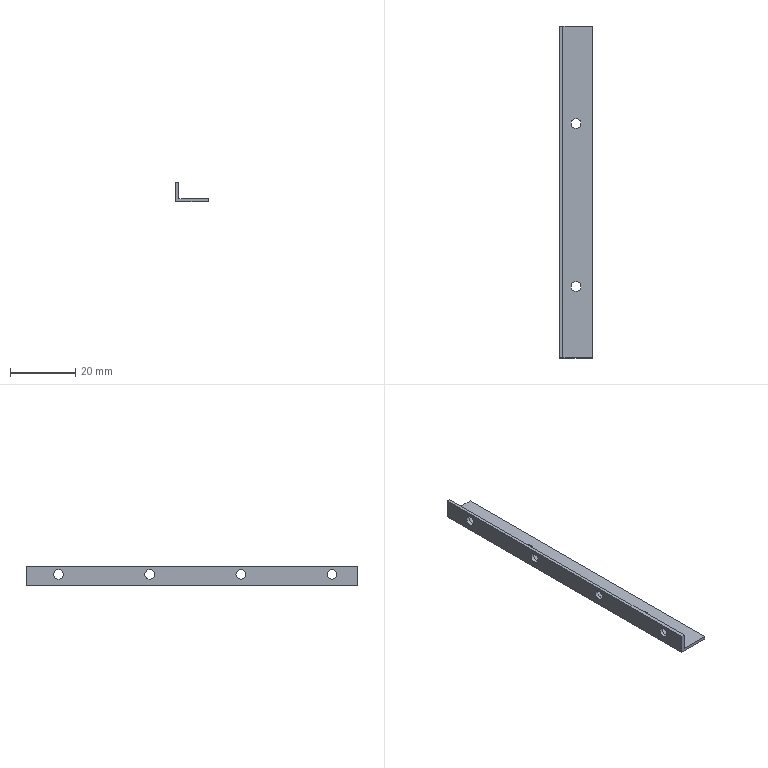Part | STEP file | 1-31.2 | 1 solid | 14 faces | box 10 x 102 x 6 mm | volume 1488 mm3 | plane 8 | cylinder 6 | commonest cylinder face diameters 3 x6
STEP:
#1=CARTESIAN_POINT('',(0.,0.,0.));
#2=DIRECTION('',(0.,0.,1.));
#3=DIRECTION('',(1.,0.,0.));
#4=AXIS2_PLACEMENT_3D('',#1,#2,#3);
#5=CARTESIAN_POINT('',(0.,-51.,0.));
#6=VERTEX_POINT('',#5);
#7=CARTESIAN_POINT('',(10.,-51.,0.));
#8=VERTEX_POINT('',#7);
#9=CARTESIAN_POINT('',(0.,-51.,0.));
#10=DIRECTION('',(1.,0.,0.));
#11=VECTOR('',#10,1.);
#12=LINE('',#9,#11);
#13=CARTESIAN_POINT('',(5.,-51.,5.));
#14=DIRECTION('',(0.,-1.,0.));
#15=DIRECTION('',(1.,0.,0.));
#16=AXIS2_PLACEMENT_3D('',#13,#14,#15);
#17=PLANE('',#16);
#18=CARTESIAN_POINT('',(-5.,-5.));
#19=DIRECTION('',(1.,0.));
#20=VECTOR('',#19,1.);
#21=LINE('',#18,#20);
#22=(GEOMETRIC_REPRESENTATION_CONTEXT(2)PARAMETRIC_REPRESENTATION_CONTEXT()REPRESENTATION_CONTEXT('',''));
#23=DEFINITIONAL_REPRESENTATION('',(#21),#22);
#24=PCURVE('',#17,#23);
#25=CARTESIAN_POINT('',(5.,0.,0.));
#26=DIRECTION('',(0.,0.,1.));
#27=DIRECTION('',(1.,0.,0.));
#28=AXIS2_PLACEMENT_3D('',#25,#26,#27);
#29=PLANE('',#28);
#30=CARTESIAN_POINT('',(-5.,-51.));
#31=DIRECTION('',(1.,0.));
#32=VECTOR('',#31,1.);
#33=LINE('',#30,#32);
#34=(GEOMETRIC_REPRESENTATION_CONTEXT(2)PARAMETRIC_REPRESENTATION_CONTEXT()REPRESENTATION_CONTEXT('',''));
#35=DEFINITIONAL_REPRESENTATION('',(#33),#34);
#36=PCURVE('',#29,#35);
#37=SURFACE_CURVE('',#12,(#24,#36),.PCURVE_S1.);
#38=EDGE_CURVE('',#6,#8,#37,.T.);
#39=ORIENTED_EDGE('',*,*,#38,.T.);
#40=CARTESIAN_POINT('',(10.,-51.,1.));
#41=VERTEX_POINT('',#40);
#42=CARTESIAN_POINT('',(10.,-51.,0.));
#43=DIRECTION('',(0.,0.,1.));
#44=VECTOR('',#43,1.);
#45=LINE('',#42,#44);
#46=CARTESIAN_POINT('',(5.,-5.));
#47=DIRECTION('',(0.,1.));
#48=VECTOR('',#47,1.);
#49=LINE('',#46,#48);
#50=(GEOMETRIC_REPRESENTATION_CONTEXT(2)PARAMETRIC_REPRESENTATION_CONTEXT()REPRESENTATION_CONTEXT('',''));
#51=DEFINITIONAL_REPRESENTATION('',(#49),#50);
#52=PCURVE('',#17,#51);
#53=CARTESIAN_POINT('',(10.,0.,0.5));
#54=DIRECTION('',(-1.,0.,0.));
#55=DIRECTION('',(0.,0.,1.));
#56=AXIS2_PLACEMENT_3D('',#53,#54,#55);
#57=PLANE('',#56);
#58=CARTESIAN_POINT('',(-0.5,-51.));
#59=DIRECTION('',(1.,0.));
#60=VECTOR('',#59,1.);
#61=LINE('',#58,#60);
#62=(GEOMETRIC_REPRESENTATION_CONTEXT(2)PARAMETRIC_REPRESENTATION_CONTEXT()REPRESENTATION_CONTEXT('',''));
#63=DEFINITIONAL_REPRESENTATION('',(#61),#62);
#64=PCURVE('',#57,#63);
#65=SURFACE_CURVE('',#45,(#52,#64),.PCURVE_S1.);
#66=EDGE_CURVE('',#8,#41,#65,.T.);
#67=ORIENTED_EDGE('',*,*,#66,.T.);
#68=CARTESIAN_POINT('',(1.,-51.,1.));
#69=VERTEX_POINT('',#68);
#70=CARTESIAN_POINT('',(10.,-51.,1.));
#71=DIRECTION('',(-1.,0.,0.));
#72=VECTOR('',#71,1.);
#73=LINE('',#70,#72);
#74=CARTESIAN_POINT('',(5.,-4.));
#75=DIRECTION('',(-1.,0.));
#76=VECTOR('',#75,1.);
#77=LINE('',#74,#76);
#78=(GEOMETRIC_REPRESENTATION_CONTEXT(2)PARAMETRIC_REPRESENTATION_CONTEXT()REPRESENTATION_CONTEXT('',''));
#79=DEFINITIONAL_REPRESENTATION('',(#77),#78);
#80=PCURVE('',#17,#79);
#81=CARTESIAN_POINT('',(5.5,0.,1.));
#82=DIRECTION('',(0.,0.,-1.));
#83=DIRECTION('',(-1.,0.,0.));
#84=AXIS2_PLACEMENT_3D('',#81,#82,#83);
#85=PLANE('',#84);
#86=CARTESIAN_POINT('',(-4.5,-51.));
#87=DIRECTION('',(1.,0.));
#88=VECTOR('',#87,1.);
#89=LINE('',#86,#88);
#90=(GEOMETRIC_REPRESENTATION_CONTEXT(2)PARAMETRIC_REPRESENTATION_CONTEXT()REPRESENTATION_CONTEXT('',''));
#91=DEFINITIONAL_REPRESENTATION('',(#89),#90);
#92=PCURVE('',#85,#91);
#93=SURFACE_CURVE('',#73,(#80,#92),.PCURVE_S1.);
#94=EDGE_CURVE('',#41,#69,#93,.T.);
#95=ORIENTED_EDGE('',*,*,#94,.T.);
#96=CARTESIAN_POINT('',(1.,-51.,6.));
#97=VERTEX_POINT('',#96);
#98=CARTESIAN_POINT('',(1.,-51.,1.));
#99=DIRECTION('',(0.,0.,1.));
#100=VECTOR('',#99,1.);
#101=LINE('',#98,#100);
#102=CARTESIAN_POINT('',(-4.,-4.));
#103=DIRECTION('',(0.,1.));
#104=VECTOR('',#103,1.);
#105=LINE('',#102,#104);
#106=(GEOMETRIC_REPRESENTATION_CONTEXT(2)PARAMETRIC_REPRESENTATION_CONTEXT()REPRESENTATION_CONTEXT('',''));
#107=DEFINITIONAL_REPRESENTATION('',(#105),#106);
#108=PCURVE('',#17,#107);
#109=CARTESIAN_POINT('',(1.,0.,3.5));
#110=DIRECTION('',(-1.,0.,0.));
#111=DIRECTION('',(0.,0.,1.));
#112=AXIS2_PLACEMENT_3D('',#109,#110,#111);
#113=PLANE('',#112);
#114=CARTESIAN_POINT('',(-2.5,-51.));
#115=DIRECTION('',(1.,0.));
#116=VECTOR('',#115,1.);
#117=LINE('',#114,#116);
#118=(GEOMETRIC_REPRESENTATION_CONTEXT(2)PARAMETRIC_REPRESENTATION_CONTEXT()REPRESENTATION_CONTEXT('',''));
#119=DEFINITIONAL_REPRESENTATION('',(#117),#118);
#120=PCURVE('',#113,#119);
#121=SURFACE_CURVE('',#101,(#108,#120),.PCURVE_S1.);
#122=EDGE_CURVE('',#69,#97,#121,.T.);
#123=ORIENTED_EDGE('',*,*,#122,.T.);
#124=CARTESIAN_POINT('',(0.,-51.,6.));
#125=VERTEX_POINT('',#124);
#126=CARTESIAN_POINT('',(1.,-51.,6.));
#127=DIRECTION('',(-1.,0.,0.));
#128=VECTOR('',#127,1.);
#129=LINE('',#126,#128);
#130=CARTESIAN_POINT('',(-4.,1.));
#131=DIRECTION('',(-1.,0.));
#132=VECTOR('',#131,1.);
#133=LINE('',#130,#132);
#134=(GEOMETRIC_REPRESENTATION_CONTEXT(2)PARAMETRIC_REPRESENTATION_CONTEXT()REPRESENTATION_CONTEXT('',''));
#135=DEFINITIONAL_REPRESENTATION('',(#133),#134);
#136=PCURVE('',#17,#135);
#137=CARTESIAN_POINT('',(0.5,0.,6.));
#138=DIRECTION('',(0.,0.,-1.));
#139=DIRECTION('',(-1.,0.,0.));
#140=AXIS2_PLACEMENT_3D('',#137,#138,#139);
#141=PLANE('',#140);
#142=CARTESIAN_POINT('',(-0.5,-51.));
#143=DIRECTION('',(1.,0.));
#144=VECTOR('',#143,1.);
#145=LINE('',#142,#144);
#146=(GEOMETRIC_REPRESENTATION_CONTEXT(2)PARAMETRIC_REPRESENTATION_CONTEXT()REPRESENTATION_CONTEXT('',''));
#147=DEFINITIONAL_REPRESENTATION('',(#145),#146);
#148=PCURVE('',#141,#147);
#149=SURFACE_CURVE('',#129,(#136,#148),.PCURVE_S1.);
#150=EDGE_CURVE('',#97,#125,#149,.T.);
#151=ORIENTED_EDGE('',*,*,#150,.T.);
#152=CARTESIAN_POINT('',(0.,-51.,6.));
#153=DIRECTION('',(0.,0.,-1.));
#154=VECTOR('',#153,1.);
#155=LINE('',#152,#154);
#156=CARTESIAN_POINT('',(-5.,1.));
#157=DIRECTION('',(0.,-1.));
#158=VECTOR('',#157,1.);
#159=LINE('',#156,#158);
#160=(GEOMETRIC_REPRESENTATION_CONTEXT(2)PARAMETRIC_REPRESENTATION_CONTEXT()REPRESENTATION_CONTEXT('',''));
#161=DEFINITIONAL_REPRESENTATION('',(#159),#160);
#162=PCURVE('',#17,#161);
#163=CARTESIAN_POINT('',(0.,0.,3.));
#164=DIRECTION('',(1.,0.,0.));
#165=DIRECTION('',(0.,0.,-1.));
#166=AXIS2_PLACEMENT_3D('',#163,#164,#165);
#167=PLANE('',#166);
#168=CARTESIAN_POINT('',(-3.,-51.));
#169=DIRECTION('',(1.,0.));
#170=VECTOR('',#169,1.);
#171=LINE('',#168,#170);
#172=(GEOMETRIC_REPRESENTATION_CONTEXT(2)PARAMETRIC_REPRESENTATION_CONTEXT()REPRESENTATION_CONTEXT('',''));
#173=DEFINITIONAL_REPRESENTATION('',(#171),#172);
#174=PCURVE('',#167,#173);
#175=SURFACE_CURVE('',#155,(#162,#174),.PCURVE_S1.);
#176=EDGE_CURVE('',#125,#6,#175,.T.);
#177=ORIENTED_EDGE('',*,*,#176,.T.);
#178=EDGE_LOOP('',(#39,#67,#95,#123,#151,#177));
#179=FACE_BOUND('',#178,.T.);
#180=ADVANCED_FACE('',(#179),#17,.T.);
#181=CARTESIAN_POINT('',(0.,51.,0.));
#182=VERTEX_POINT('',#181);
#183=CARTESIAN_POINT('',(10.,51.,0.));
#184=VERTEX_POINT('',#183);
#185=CARTESIAN_POINT('',(0.,51.,0.));
#186=DIRECTION('',(1.,0.,0.));
#187=VECTOR('',#186,1.);
#188=LINE('',#185,#187);
#189=CARTESIAN_POINT('',(5.,51.,5.));
#190=DIRECTION('',(0.,-1.,0.));
#191=DIRECTION('',(1.,0.,0.));
#192=AXIS2_PLACEMENT_3D('',#189,#190,#191);
#193=PLANE('',#192);
#194=CARTESIAN_POINT('',(-5.,-5.));
#195=DIRECTION('',(1.,0.));
#196=VECTOR('',#195,1.);
#197=LINE('',#194,#196);
#198=(GEOMETRIC_REPRESENTATION_CONTEXT(2)PARAMETRIC_REPRESENTATION_CONTEXT()REPRESENTATION_CONTEXT('',''));
#199=DEFINITIONAL_REPRESENTATION('',(#197),#198);
#200=PCURVE('',#193,#199);
#201=CARTESIAN_POINT('',(-5.,51.));
#202=DIRECTION('',(1.,0.));
#203=VECTOR('',#202,1.);
#204=LINE('',#201,#203);
#205=(GEOMETRIC_REPRESENTATION_CONTEXT(2)PARAMETRIC_REPRESENTATION_CONTEXT()REPRESENTATION_CONTEXT('',''));
#206=DEFINITIONAL_REPRESENTATION('',(#204),#205);
#207=PCURVE('',#29,#206);
#208=SURFACE_CURVE('',#188,(#200,#207),.PCURVE_S1.);
#209=EDGE_CURVE('',#182,#184,#208,.T.);
#210=ORIENTED_EDGE('',*,*,#209,.T.);
#211=CARTESIAN_POINT('',(10.,51.,1.));
#212=VERTEX_POINT('',#211);
#213=CARTESIAN_POINT('',(10.,51.,0.));
#214=DIRECTION('',(0.,0.,1.));
#215=VECTOR('',#214,1.);
#216=LINE('',#213,#215);
#217=CARTESIAN_POINT('',(5.,-5.));
#218=DIRECTION('',(0.,1.));
#219=VECTOR('',#218,1.);
#220=LINE('',#217,#219);
#221=(GEOMETRIC_REPRESENTATION_CONTEXT(2)PARAMETRIC_REPRESENTATION_CONTEXT()REPRESENTATION_CONTEXT('',''));
#222=DEFINITIONAL_REPRESENTATION('',(#220),#221);
#223=PCURVE('',#193,#222);
#224=CARTESIAN_POINT('',(-0.5,51.));
#225=DIRECTION('',(1.,0.));
#226=VECTOR('',#225,1.);
#227=LINE('',#224,#226);
#228=(GEOMETRIC_REPRESENTATION_CONTEXT(2)PARAMETRIC_REPRESENTATION_CONTEXT()REPRESENTATION_CONTEXT('',''));
#229=DEFINITIONAL_REPRESENTATION('',(#227),#228);
#230=PCURVE('',#57,#229);
#231=SURFACE_CURVE('',#216,(#223,#230),.PCURVE_S1.);
#232=EDGE_CURVE('',#184,#212,#231,.T.);
#233=ORIENTED_EDGE('',*,*,#232,.T.);
#234=CARTESIAN_POINT('',(1.,51.,1.));
#235=VERTEX_POINT('',#234);
#236=CARTESIAN_POINT('',(10.,51.,1.));
#237=DIRECTION('',(-1.,0.,0.));
#238=VECTOR('',#237,1.);
#239=LINE('',#236,#238);
#240=CARTESIAN_POINT('',(5.,-4.));
#241=DIRECTION('',(-1.,0.));
#242=VECTOR('',#241,1.);
#243=LINE('',#240,#242);
#244=(GEOMETRIC_REPRESENTATION_CONTEXT(2)PARAMETRIC_REPRESENTATION_CONTEXT()REPRESENTATION_CONTEXT('',''));
#245=DEFINITIONAL_REPRESENTATION('',(#243),#244);
#246=PCURVE('',#193,#245);
#247=CARTESIAN_POINT('',(-4.5,51.));
#248=DIRECTION('',(1.,0.));
#249=VECTOR('',#248,1.);
#250=LINE('',#247,#249);
#251=(GEOMETRIC_REPRESENTATION_CONTEXT(2)PARAMETRIC_REPRESENTATION_CONTEXT()REPRESENTATION_CONTEXT('',''));
#252=DEFINITIONAL_REPRESENTATION('',(#250),#251);
#253=PCURVE('',#85,#252);
#254=SURFACE_CURVE('',#239,(#246,#253),.PCURVE_S1.);
#255=EDGE_CURVE('',#212,#235,#254,.T.);
#256=ORIENTED_EDGE('',*,*,#255,.T.);
#257=CARTESIAN_POINT('',(1.,51.,6.));
#258=VERTEX_POINT('',#257);
#259=CARTESIAN_POINT('',(1.,51.,1.));
#260=DIRECTION('',(0.,0.,1.));
#261=VECTOR('',#260,1.);
#262=LINE('',#259,#261);
#263=CARTESIAN_POINT('',(-4.,-4.));
#264=DIRECTION('',(0.,1.));
#265=VECTOR('',#264,1.);
#266=LINE('',#263,#265);
#267=(GEOMETRIC_REPRESENTATION_CONTEXT(2)PARAMETRIC_REPRESENTATION_CONTEXT()REPRESENTATION_CONTEXT('',''));
#268=DEFINITIONAL_REPRESENTATION('',(#266),#267);
#269=PCURVE('',#193,#268);
#270=CARTESIAN_POINT('',(-2.5,51.));
#271=DIRECTION('',(1.,0.));
#272=VECTOR('',#271,1.);
#273=LINE('',#270,#272);
#274=(GEOMETRIC_REPRESENTATION_CONTEXT(2)PARAMETRIC_REPRESENTATION_CONTEXT()REPRESENTATION_CONTEXT('',''));
#275=DEFINITIONAL_REPRESENTATION('',(#273),#274);
#276=PCURVE('',#113,#275);
#277=SURFACE_CURVE('',#262,(#269,#276),.PCURVE_S1.);
#278=EDGE_CURVE('',#235,#258,#277,.T.);
#279=ORIENTED_EDGE('',*,*,#278,.T.);
#280=CARTESIAN_POINT('',(0.,51.,6.));
#281=VERTEX_POINT('',#280);
#282=CARTESIAN_POINT('',(1.,51.,6.));
#283=DIRECTION('',(-1.,0.,0.));
#284=VECTOR('',#283,1.);
#285=LINE('',#282,#284);
#286=CARTESIAN_POINT('',(-4.,1.));
#287=DIRECTION('',(-1.,0.));
#288=VECTOR('',#287,1.);
#289=LINE('',#286,#288);
#290=(GEOMETRIC_REPRESENTATION_CONTEXT(2)PARAMETRIC_REPRESENTATION_CONTEXT()REPRESENTATION_CONTEXT('',''));
#291=DEFINITIONAL_REPRESENTATION('',(#289),#290);
#292=PCURVE('',#193,#291);
#293=CARTESIAN_POINT('',(-0.5,51.));
#294=DIRECTION('',(1.,0.));
#295=VECTOR('',#294,1.);
#296=LINE('',#293,#295);
#297=(GEOMETRIC_REPRESENTATION_CONTEXT(2)PARAMETRIC_REPRESENTATION_CONTEXT()REPRESENTATION_CONTEXT('',''));
#298=DEFINITIONAL_REPRESENTATION('',(#296),#297);
#299=PCURVE('',#141,#298);
#300=SURFACE_CURVE('',#285,(#292,#299),.PCURVE_S1.);
#301=EDGE_CURVE('',#258,#281,#300,.T.);
#302=ORIENTED_EDGE('',*,*,#301,.T.);
#303=CARTESIAN_POINT('',(0.,51.,6.));
#304=DIRECTION('',(0.,0.,-1.));
#305=VECTOR('',#304,1.);
#306=LINE('',#303,#305);
#307=CARTESIAN_POINT('',(-5.,1.));
#308=DIRECTION('',(0.,-1.));
#309=VECTOR('',#308,1.);
#310=LINE('',#307,#309);
#311=(GEOMETRIC_REPRESENTATION_CONTEXT(2)PARAMETRIC_REPRESENTATION_CONTEXT()REPRESENTATION_CONTEXT('',''));
#312=DEFINITIONAL_REPRESENTATION('',(#310),#311);
#313=PCURVE('',#193,#312);
#314=CARTESIAN_POINT('',(-3.,51.));
#315=DIRECTION('',(1.,0.));
#316=VECTOR('',#315,1.);
#317=LINE('',#314,#316);
#318=(GEOMETRIC_REPRESENTATION_CONTEXT(2)PARAMETRIC_REPRESENTATION_CONTEXT()REPRESENTATION_CONTEXT('',''));
#319=DEFINITIONAL_REPRESENTATION('',(#317),#318);
#320=PCURVE('',#167,#319);
#321=SURFACE_CURVE('',#306,(#313,#320),.PCURVE_S1.);
#322=EDGE_CURVE('',#281,#182,#321,.T.);
#323=ORIENTED_EDGE('',*,*,#322,.T.);
#324=EDGE_LOOP('',(#210,#233,#256,#279,#302,#323));
#325=FACE_BOUND('',#324,.F.);
#326=ADVANCED_FACE('',(#325),#193,.F.);
#327=ORIENTED_EDGE('',*,*,#66,.T.);
#328=CARTESIAN_POINT('',(10.,-51.,1.));
#329=DIRECTION('',(0.,1.,0.));
#330=VECTOR('',#329,1.);
#331=LINE('',#328,#330);
#332=CARTESIAN_POINT('',(0.5,-51.));
#333=DIRECTION('',(0.,1.));
#334=VECTOR('',#333,1.);
#335=LINE('',#332,#334);
#336=(GEOMETRIC_REPRESENTATION_CONTEXT(2)PARAMETRIC_REPRESENTATION_CONTEXT()REPRESENTATION_CONTEXT('',''));
#337=DEFINITIONAL_REPRESENTATION('',(#335),#336);
#338=PCURVE('',#57,#337);
#339=CARTESIAN_POINT('',(-4.5,-51.));
#340=DIRECTION('',(0.,1.));
#341=VECTOR('',#340,1.);
#342=LINE('',#339,#341);
#343=(GEOMETRIC_REPRESENTATION_CONTEXT(2)PARAMETRIC_REPRESENTATION_CONTEXT()REPRESENTATION_CONTEXT('',''));
#344=DEFINITIONAL_REPRESENTATION('',(#342),#343);
#345=PCURVE('',#85,#344);
#346=SURFACE_CURVE('',#331,(#338,#345),.PCURVE_S1.);
#347=EDGE_CURVE('',#41,#212,#346,.T.);
#348=ORIENTED_EDGE('',*,*,#347,.T.);
#349=ORIENTED_EDGE('',*,*,#232,.F.);
#350=CARTESIAN_POINT('',(10.,-51.,0.));
#351=DIRECTION('',(0.,1.,0.));
#352=VECTOR('',#351,1.);
#353=LINE('',#350,#352);
#354=CARTESIAN_POINT('',(-0.5,-51.));
#355=DIRECTION('',(0.,1.));
#356=VECTOR('',#355,1.);
#357=LINE('',#354,#356);
#358=(GEOMETRIC_REPRESENTATION_CONTEXT(2)PARAMETRIC_REPRESENTATION_CONTEXT()REPRESENTATION_CONTEXT('',''));
#359=DEFINITIONAL_REPRESENTATION('',(#357),#358);
#360=PCURVE('',#57,#359);
#361=CARTESIAN_POINT('',(5.,-51.));
#362=DIRECTION('',(0.,1.));
#363=VECTOR('',#362,1.);
#364=LINE('',#361,#363);
#365=(GEOMETRIC_REPRESENTATION_CONTEXT(2)PARAMETRIC_REPRESENTATION_CONTEXT()REPRESENTATION_CONTEXT('',''));
#366=DEFINITIONAL_REPRESENTATION('',(#364),#365);
#367=PCURVE('',#29,#366);
#368=SURFACE_CURVE('',#353,(#360,#367),.PCURVE_S1.);
#369=EDGE_CURVE('',#8,#184,#368,.T.);
#370=ORIENTED_EDGE('',*,*,#369,.F.);
#371=EDGE_LOOP('',(#327,#348,#349,#370));
#372=FACE_BOUND('',#371,.F.);
#373=ADVANCED_FACE('',(#372),#57,.F.);
#374=ORIENTED_EDGE('',*,*,#150,.T.);
#375=CARTESIAN_POINT('',(0.,-51.,6.));
#376=DIRECTION('',(0.,1.,0.));
#377=VECTOR('',#376,1.);
#378=LINE('',#375,#377);
#379=CARTESIAN_POINT('',(0.5,-51.));
#380=DIRECTION('',(0.,1.));
#381=VECTOR('',#380,1.);
#382=LINE('',#379,#381);
#383=(GEOMETRIC_REPRESENTATION_CONTEXT(2)PARAMETRIC_REPRESENTATION_CONTEXT()REPRESENTATION_CONTEXT('',''));
#384=DEFINITIONAL_REPRESENTATION('',(#382),#383);
#385=PCURVE('',#141,#384);
#386=CARTESIAN_POINT('',(-3.,-51.));
#387=DIRECTION('',(0.,1.));
#388=VECTOR('',#387,1.);
#389=LINE('',#386,#388);
#390=(GEOMETRIC_REPRESENTATION_CONTEXT(2)PARAMETRIC_REPRESENTATION_CONTEXT()REPRESENTATION_CONTEXT('',''));
#391=DEFINITIONAL_REPRESENTATION('',(#389),#390);
#392=PCURVE('',#167,#391);
#393=SURFACE_CURVE('',#378,(#385,#392),.PCURVE_S1.);
#394=EDGE_CURVE('',#125,#281,#393,.T.);
#395=ORIENTED_EDGE('',*,*,#394,.T.);
#396=ORIENTED_EDGE('',*,*,#301,.F.);
#397=CARTESIAN_POINT('',(1.,-51.,6.));
#398=DIRECTION('',(0.,1.,0.));
#399=VECTOR('',#398,1.);
#400=LINE('',#397,#399);
#401=CARTESIAN_POINT('',(-0.5,-51.));
#402=DIRECTION('',(0.,1.));
#403=VECTOR('',#402,1.);
#404=LINE('',#401,#403);
#405=(GEOMETRIC_REPRESENTATION_CONTEXT(2)PARAMETRIC_REPRESENTATION_CONTEXT()REPRESENTATION_CONTEXT('',''));
#406=DEFINITIONAL_REPRESENTATION('',(#404),#405);
#407=PCURVE('',#141,#406);
#408=CARTESIAN_POINT('',(2.5,-51.));
#409=DIRECTION('',(0.,1.));
#410=VECTOR('',#409,1.);
#411=LINE('',#408,#410);
#412=(GEOMETRIC_REPRESENTATION_CONTEXT(2)PARAMETRIC_REPRESENTATION_CONTEXT()REPRESENTATION_CONTEXT('',''));
#413=DEFINITIONAL_REPRESENTATION('',(#411),#412);
#414=PCURVE('',#113,#413);
#415=SURFACE_CURVE('',#400,(#407,#414),.PCURVE_S1.);
#416=EDGE_CURVE('',#97,#258,#415,.T.);
#417=ORIENTED_EDGE('',*,*,#416,.F.);
#418=EDGE_LOOP('',(#374,#395,#396,#417));
#419=FACE_BOUND('',#418,.F.);
#420=ADVANCED_FACE('',(#419),#141,.F.);
#421=ORIENTED_EDGE('',*,*,#122,.T.);
#422=ORIENTED_EDGE('',*,*,#416,.T.);
#423=ORIENTED_EDGE('',*,*,#278,.F.);
#424=CARTESIAN_POINT('',(1.,-51.,1.));
#425=DIRECTION('',(0.,1.,0.));
#426=VECTOR('',#425,1.);
#427=LINE('',#424,#426);
#428=CARTESIAN_POINT('',(-2.5,-51.));
#429=DIRECTION('',(0.,1.));
#430=VECTOR('',#429,1.);
#431=LINE('',#428,#430);
#432=(GEOMETRIC_REPRESENTATION_CONTEXT(2)PARAMETRIC_REPRESENTATION_CONTEXT()REPRESENTATION_CONTEXT('',''));
#433=DEFINITIONAL_REPRESENTATION('',(#431),#432);
#434=PCURVE('',#113,#433);
#435=CARTESIAN_POINT('',(4.5,-51.));
#436=DIRECTION('',(0.,1.));
#437=VECTOR('',#436,1.);
#438=LINE('',#435,#437);
#439=(GEOMETRIC_REPRESENTATION_CONTEXT(2)PARAMETRIC_REPRESENTATION_CONTEXT()REPRESENTATION_CONTEXT('',''));
#440=DEFINITIONAL_REPRESENTATION('',(#438),#439);
#441=PCURVE('',#85,#440);
#442=SURFACE_CURVE('',#427,(#434,#441),.PCURVE_S1.);
#443=EDGE_CURVE('',#69,#235,#442,.T.);
#444=ORIENTED_EDGE('',*,*,#443,.F.);
#445=EDGE_LOOP('',(#421,#422,#423,#444));
#446=FACE_BOUND('',#445,.F.);
#447=CARTESIAN_POINT('',(1.,42.5,3.5));
#448=VERTEX_POINT('',#447);
#449=CARTESIAN_POINT('',(1.,41.,3.5));
#450=DIRECTION('',(1.,0.,0.));
#451=DIRECTION('',(0.,1.,0.));
#452=AXIS2_PLACEMENT_3D('',#449,#450,#451);
#453=CIRCLE('',#452,1.5);
#454=CARTESIAN_POINT('',(0.,42.5));
#455=CARTESIAN_POINT('',(2.598,42.5));
#456=CARTESIAN_POINT('',(1.299,40.25));
#457=CARTESIAN_POINT('',(0.,38.));
#458=CARTESIAN_POINT('',(-1.299,40.25));
#459=CARTESIAN_POINT('',(-2.598,42.5));
#460=CARTESIAN_POINT('',(0.,42.5));
#461=(BOUNDED_CURVE()B_SPLINE_CURVE(2,(#454,#455,#456,#457,#458,#459,#460),.UNSPECIFIED.,.T.,.F.)B_SPLINE_CURVE_WITH_KNOTS((1,2,2,2,2,1),(-2.094,0.,2.094,4.189,6.283,8.378),.UNSPECIFIED.)CURVE()GEOMETRIC_REPRESENTATION_ITEM()RATIONAL_B_SPLINE_CURVE((1.,0.5,1.,0.5,1.,0.5,1.))REPRESENTATION_ITEM(''));
#462=(GEOMETRIC_REPRESENTATION_CONTEXT(2)PARAMETRIC_REPRESENTATION_CONTEXT()REPRESENTATION_CONTEXT('',''));
#463=DEFINITIONAL_REPRESENTATION('',(#461),#462);
#464=PCURVE('',#113,#463);
#465=CARTESIAN_POINT('',(52.,41.,3.5));
#466=DIRECTION('',(-1.,0.,0.));
#467=DIRECTION('',(0.,1.,0.));
#468=AXIS2_PLACEMENT_3D('',#465,#466,#467);
#469=CYLINDRICAL_SURFACE('',#468,1.5);
#470=CARTESIAN_POINT('',(6.283,51.));
#471=DIRECTION('',(-1.,0.));
#472=VECTOR('',#471,1.);
#473=LINE('',#470,#472);
#474=(GEOMETRIC_REPRESENTATION_CONTEXT(2)PARAMETRIC_REPRESENTATION_CONTEXT()REPRESENTATION_CONTEXT('',''));
#475=DEFINITIONAL_REPRESENTATION('',(#473),#474);
#476=PCURVE('',#469,#475);
#477=SURFACE_CURVE('',#453,(#464,#476),.PCURVE_S1.);
#478=EDGE_CURVE('',#448,#448,#477,.T.);
#479=ORIENTED_EDGE('',*,*,#478,.T.);
#480=EDGE_LOOP('',(#479));
#481=FACE_BOUND('',#480,.F.);
#482=CARTESIAN_POINT('',(1.,14.5,3.5));
#483=VERTEX_POINT('',#482);
#484=CARTESIAN_POINT('',(1.,13.,3.5));
#485=DIRECTION('',(1.,0.,0.));
#486=DIRECTION('',(0.,1.,0.));
#487=AXIS2_PLACEMENT_3D('',#484,#485,#486);
#488=CIRCLE('',#487,1.5);
#489=CARTESIAN_POINT('',(0.,14.5));
#490=CARTESIAN_POINT('',(2.598,14.5));
#491=CARTESIAN_POINT('',(1.299,12.25));
#492=CARTESIAN_POINT('',(0.,10.));
#493=CARTESIAN_POINT('',(-1.299,12.25));
#494=CARTESIAN_POINT('',(-2.598,14.5));
#495=CARTESIAN_POINT('',(0.,14.5));
#496=(BOUNDED_CURVE()B_SPLINE_CURVE(2,(#489,#490,#491,#492,#493,#494,#495),.UNSPECIFIED.,.T.,.F.)B_SPLINE_CURVE_WITH_KNOTS((1,2,2,2,2,1),(-2.094,0.,2.094,4.189,6.283,8.378),.UNSPECIFIED.)CURVE()GEOMETRIC_REPRESENTATION_ITEM()RATIONAL_B_SPLINE_CURVE((1.,0.5,1.,0.5,1.,0.5,1.))REPRESENTATION_ITEM(''));
#497=(GEOMETRIC_REPRESENTATION_CONTEXT(2)PARAMETRIC_REPRESENTATION_CONTEXT()REPRESENTATION_CONTEXT('',''));
#498=DEFINITIONAL_REPRESENTATION('',(#496),#497);
#499=PCURVE('',#113,#498);
#500=CARTESIAN_POINT('',(52.,13.,3.5));
#501=DIRECTION('',(-1.,0.,0.));
#502=DIRECTION('',(0.,1.,0.));
#503=AXIS2_PLACEMENT_3D('',#500,#501,#502);
#504=CYLINDRICAL_SURFACE('',#503,1.5);
#505=CARTESIAN_POINT('',(6.283,51.));
#506=DIRECTION('',(-1.,0.));
#507=VECTOR('',#506,1.);
#508=LINE('',#505,#507);
#509=(GEOMETRIC_REPRESENTATION_CONTEXT(2)PARAMETRIC_REPRESENTATION_CONTEXT()REPRESENTATION_CONTEXT('',''));
#510=DEFINITIONAL_REPRESENTATION('',(#508),#509);
#511=PCURVE('',#504,#510);
#512=SURFACE_CURVE('',#488,(#499,#511),.PCURVE_S1.);
#513=EDGE_CURVE('',#483,#483,#512,.T.);
#514=ORIENTED_EDGE('',*,*,#513,.T.);
#515=EDGE_LOOP('',(#514));
#516=FACE_BOUND('',#515,.F.);
#517=CARTESIAN_POINT('',(1.,-41.5,3.5));
#518=VERTEX_POINT('',#517);
#519=CARTESIAN_POINT('',(1.,-43.,3.5));
#520=DIRECTION('',(1.,0.,0.));
#521=DIRECTION('',(0.,1.,0.));
#522=AXIS2_PLACEMENT_3D('',#519,#520,#521);
#523=CIRCLE('',#522,1.5);
#524=CARTESIAN_POINT('',(0.,-41.5));
#525=CARTESIAN_POINT('',(2.598,-41.5));
#526=CARTESIAN_POINT('',(1.299,-43.75));
#527=CARTESIAN_POINT('',(0.,-46.));
#528=CARTESIAN_POINT('',(-1.299,-43.75));
#529=CARTESIAN_POINT('',(-2.598,-41.5));
#530=CARTESIAN_POINT('',(0.,-41.5));
#531=(BOUNDED_CURVE()B_SPLINE_CURVE(2,(#524,#525,#526,#527,#528,#529,#530),.UNSPECIFIED.,.T.,.F.)B_SPLINE_CURVE_WITH_KNOTS((1,2,2,2,2,1),(-2.094,0.,2.094,4.189,6.283,8.378),.UNSPECIFIED.)CURVE()GEOMETRIC_REPRESENTATION_ITEM()RATIONAL_B_SPLINE_CURVE((1.,0.5,1.,0.5,1.,0.5,1.))REPRESENTATION_ITEM(''));
#532=(GEOMETRIC_REPRESENTATION_CONTEXT(2)PARAMETRIC_REPRESENTATION_CONTEXT()REPRESENTATION_CONTEXT('',''));
#533=DEFINITIONAL_REPRESENTATION('',(#531),#532);
#534=PCURVE('',#113,#533);
#535=CARTESIAN_POINT('',(52.,-43.,3.5));
#536=DIRECTION('',(-1.,0.,0.));
#537=DIRECTION('',(0.,1.,0.));
#538=AXIS2_PLACEMENT_3D('',#535,#536,#537);
#539=CYLINDRICAL_SURFACE('',#538,1.5);
#540=CARTESIAN_POINT('',(6.283,51.));
#541=DIRECTION('',(-1.,0.));
#542=VECTOR('',#541,1.);
#543=LINE('',#540,#542);
#544=(GEOMETRIC_REPRESENTATION_CONTEXT(2)PARAMETRIC_REPRESENTATION_CONTEXT()REPRESENTATION_CONTEXT('',''));
#545=DEFINITIONAL_REPRESENTATION('',(#543),#544);
#546=PCURVE('',#539,#545);
#547=SURFACE_CURVE('',#523,(#534,#546),.PCURVE_S1.);
#548=EDGE_CURVE('',#518,#518,#547,.T.);
#549=ORIENTED_EDGE('',*,*,#548,.T.);
#550=EDGE_LOOP('',(#549));
#551=FACE_BOUND('',#550,.F.);
#552=CARTESIAN_POINT('',(1.,-13.5,3.5));
#553=VERTEX_POINT('',#552);
#554=CARTESIAN_POINT('',(1.,-15.,3.5));
#555=DIRECTION('',(1.,0.,0.));
#556=DIRECTION('',(0.,1.,0.));
#557=AXIS2_PLACEMENT_3D('',#554,#555,#556);
#558=CIRCLE('',#557,1.5);
#559=CARTESIAN_POINT('',(0.,-13.5));
#560=CARTESIAN_POINT('',(2.598,-13.5));
#561=CARTESIAN_POINT('',(1.299,-15.75));
#562=CARTESIAN_POINT('',(0.,-18.));
#563=CARTESIAN_POINT('',(-1.299,-15.75));
#564=CARTESIAN_POINT('',(-2.598,-13.5));
#565=CARTESIAN_POINT('',(0.,-13.5));
#566=(BOUNDED_CURVE()B_SPLINE_CURVE(2,(#559,#560,#561,#562,#563,#564,#565),.UNSPECIFIED.,.T.,.F.)B_SPLINE_CURVE_WITH_KNOTS((1,2,2,2,2,1),(-2.094,0.,2.094,4.189,6.283,8.378),.UNSPECIFIED.)CURVE()GEOMETRIC_REPRESENTATION_ITEM()RATIONAL_B_SPLINE_CURVE((1.,0.5,1.,0.5,1.,0.5,1.))REPRESENTATION_ITEM(''));
#567=(GEOMETRIC_REPRESENTATION_CONTEXT(2)PARAMETRIC_REPRESENTATION_CONTEXT()REPRESENTATION_CONTEXT('',''));
#568=DEFINITIONAL_REPRESENTATION('',(#566),#567);
#569=PCURVE('',#113,#568);
#570=CARTESIAN_POINT('',(52.,-15.,3.5));
#571=DIRECTION('',(-1.,0.,0.));
#572=DIRECTION('',(0.,1.,0.));
#573=AXIS2_PLACEMENT_3D('',#570,#571,#572);
#574=CYLINDRICAL_SURFACE('',#573,1.5);
#575=CARTESIAN_POINT('',(6.283,51.));
#576=DIRECTION('',(-1.,0.));
#577=VECTOR('',#576,1.);
#578=LINE('',#575,#577);
#579=(GEOMETRIC_REPRESENTATION_CONTEXT(2)PARAMETRIC_REPRESENTATION_CONTEXT()REPRESENTATION_CONTEXT('',''));
#580=DEFINITIONAL_REPRESENTATION('',(#578),#579);
#581=PCURVE('',#574,#580);
#582=SURFACE_CURVE('',#558,(#569,#581),.PCURVE_S1.);
#583=EDGE_CURVE('',#553,#553,#582,.T.);
#584=ORIENTED_EDGE('',*,*,#583,.T.);
#585=EDGE_LOOP('',(#584));
#586=FACE_BOUND('',#585,.F.);
#587=ADVANCED_FACE('',(#446,#481,#516,#551,#586),#113,.F.);
#588=ORIENTED_EDGE('',*,*,#176,.T.);
#589=CARTESIAN_POINT('',(0.,-51.,0.));
#590=DIRECTION('',(0.,1.,0.));
#591=VECTOR('',#590,1.);
#592=LINE('',#589,#591);
#593=CARTESIAN_POINT('',(3.,-51.));
#594=DIRECTION('',(0.,1.));
#595=VECTOR('',#594,1.);
#596=LINE('',#593,#595);
#597=(GEOMETRIC_REPRESENTATION_CONTEXT(2)PARAMETRIC_REPRESENTATION_CONTEXT()REPRESENTATION_CONTEXT('',''));
#598=DEFINITIONAL_REPRESENTATION('',(#596),#597);
#599=PCURVE('',#167,#598);
#600=CARTESIAN_POINT('',(-5.,-51.));
#601=DIRECTION('',(0.,1.));
#602=VECTOR('',#601,1.);
#603=LINE('',#600,#602);
#604=(GEOMETRIC_REPRESENTATION_CONTEXT(2)PARAMETRIC_REPRESENTATION_CONTEXT()REPRESENTATION_CONTEXT('',''));
#605=DEFINITIONAL_REPRESENTATION('',(#603),#604);
#606=PCURVE('',#29,#605);
#607=SURFACE_CURVE('',#592,(#599,#606),.PCURVE_S1.);
#608=EDGE_CURVE('',#6,#182,#607,.T.);
#609=ORIENTED_EDGE('',*,*,#608,.T.);
#610=ORIENTED_EDGE('',*,*,#322,.F.);
#611=ORIENTED_EDGE('',*,*,#394,.F.);
#612=EDGE_LOOP('',(#588,#609,#610,#611));
#613=FACE_BOUND('',#612,.F.);
#614=CARTESIAN_POINT('',(0.,42.5,3.5));
#615=VERTEX_POINT('',#614);
#616=CARTESIAN_POINT('',(0.,41.,3.5));
#617=DIRECTION('',(-1.,0.,0.));
#618=DIRECTION('',(0.,1.,0.));
#619=AXIS2_PLACEMENT_3D('',#616,#617,#618);
#620=CIRCLE('',#619,1.5);
#621=CARTESIAN_POINT('',(-0.5,42.5));
#622=CARTESIAN_POINT('',(2.098,42.5));
#623=CARTESIAN_POINT('',(0.799,40.25));
#624=CARTESIAN_POINT('',(-0.5,38.));
#625=CARTESIAN_POINT('',(-1.799,40.25));
#626=CARTESIAN_POINT('',(-3.098,42.5));
#627=CARTESIAN_POINT('',(-0.5,42.5));
#628=(BOUNDED_CURVE()B_SPLINE_CURVE(2,(#621,#622,#623,#624,#625,#626,#627),.UNSPECIFIED.,.T.,.F.)B_SPLINE_CURVE_WITH_KNOTS((1,2,2,2,2,1),(-2.094,0.,2.094,4.189,6.283,8.378),.UNSPECIFIED.)CURVE()GEOMETRIC_REPRESENTATION_ITEM()RATIONAL_B_SPLINE_CURVE((1.,0.5,1.,0.5,1.,0.5,1.))REPRESENTATION_ITEM(''));
#629=(GEOMETRIC_REPRESENTATION_CONTEXT(2)PARAMETRIC_REPRESENTATION_CONTEXT()REPRESENTATION_CONTEXT('',''));
#630=DEFINITIONAL_REPRESENTATION('',(#628),#629);
#631=PCURVE('',#167,#630);
#632=CARTESIAN_POINT('',(0.,52.));
#633=DIRECTION('',(1.,0.));
#634=VECTOR('',#633,1.);
#635=LINE('',#632,#634);
#636=(GEOMETRIC_REPRESENTATION_CONTEXT(2)PARAMETRIC_REPRESENTATION_CONTEXT()REPRESENTATION_CONTEXT('',''));
#637=DEFINITIONAL_REPRESENTATION('',(#635),#636);
#638=PCURVE('',#469,#637);
#639=SURFACE_CURVE('',#620,(#631,#638),.PCURVE_S1.);
#640=EDGE_CURVE('',#615,#615,#639,.T.);
#641=ORIENTED_EDGE('',*,*,#640,.T.);
#642=EDGE_LOOP('',(#641));
#643=FACE_BOUND('',#642,.F.);
#644=CARTESIAN_POINT('',(0.,14.5,3.5));
#645=VERTEX_POINT('',#644);
#646=CARTESIAN_POINT('',(0.,13.,3.5));
#647=DIRECTION('',(-1.,0.,0.));
#648=DIRECTION('',(0.,1.,0.));
#649=AXIS2_PLACEMENT_3D('',#646,#647,#648);
#650=CIRCLE('',#649,1.5);
#651=CARTESIAN_POINT('',(-0.5,14.5));
#652=CARTESIAN_POINT('',(2.098,14.5));
#653=CARTESIAN_POINT('',(0.799,12.25));
#654=CARTESIAN_POINT('',(-0.5,10.));
#655=CARTESIAN_POINT('',(-1.799,12.25));
#656=CARTESIAN_POINT('',(-3.098,14.5));
#657=CARTESIAN_POINT('',(-0.5,14.5));
#658=(BOUNDED_CURVE()B_SPLINE_CURVE(2,(#651,#652,#653,#654,#655,#656,#657),.UNSPECIFIED.,.T.,.F.)B_SPLINE_CURVE_WITH_KNOTS((1,2,2,2,2,1),(-2.094,0.,2.094,4.189,6.283,8.378),.UNSPECIFIED.)CURVE()GEOMETRIC_REPRESENTATION_ITEM()RATIONAL_B_SPLINE_CURVE((1.,0.5,1.,0.5,1.,0.5,1.))REPRESENTATION_ITEM(''));
#659=(GEOMETRIC_REPRESENTATION_CONTEXT(2)PARAMETRIC_REPRESENTATION_CONTEXT()REPRESENTATION_CONTEXT('',''));
#660=DEFINITIONAL_REPRESENTATION('',(#658),#659);
#661=PCURVE('',#167,#660);
#662=CARTESIAN_POINT('',(0.,52.));
#663=DIRECTION('',(1.,0.));
#664=VECTOR('',#663,1.);
#665=LINE('',#662,#664);
#666=(GEOMETRIC_REPRESENTATION_CONTEXT(2)PARAMETRIC_REPRESENTATION_CONTEXT()REPRESENTATION_CONTEXT('',''));
#667=DEFINITIONAL_REPRESENTATION('',(#665),#666);
#668=PCURVE('',#504,#667);
#669=SURFACE_CURVE('',#650,(#661,#668),.PCURVE_S1.);
#670=EDGE_CURVE('',#645,#645,#669,.T.);
#671=ORIENTED_EDGE('',*,*,#670,.T.);
#672=EDGE_LOOP('',(#671));
#673=FACE_BOUND('',#672,.F.);
#674=CARTESIAN_POINT('',(0.,-41.5,3.5));
#675=VERTEX_POINT('',#674);
#676=CARTESIAN_POINT('',(0.,-43.,3.5));
#677=DIRECTION('',(-1.,0.,0.));
#678=DIRECTION('',(0.,1.,0.));
#679=AXIS2_PLACEMENT_3D('',#676,#677,#678);
#680=CIRCLE('',#679,1.5);
#681=CARTESIAN_POINT('',(-0.5,-41.5));
#682=CARTESIAN_POINT('',(2.098,-41.5));
#683=CARTESIAN_POINT('',(0.799,-43.75));
#684=CARTESIAN_POINT('',(-0.5,-46.));
#685=CARTESIAN_POINT('',(-1.799,-43.75));
#686=CARTESIAN_POINT('',(-3.098,-41.5));
#687=CARTESIAN_POINT('',(-0.5,-41.5));
#688=(BOUNDED_CURVE()B_SPLINE_CURVE(2,(#681,#682,#683,#684,#685,#686,#687),.UNSPECIFIED.,.T.,.F.)B_SPLINE_CURVE_WITH_KNOTS((1,2,2,2,2,1),(-2.094,0.,2.094,4.189,6.283,8.378),.UNSPECIFIED.)CURVE()GEOMETRIC_REPRESENTATION_ITEM()RATIONAL_B_SPLINE_CURVE((1.,0.5,1.,0.5,1.,0.5,1.))REPRESENTATION_ITEM(''));
#689=(GEOMETRIC_REPRESENTATION_CONTEXT(2)PARAMETRIC_REPRESENTATION_CONTEXT()REPRESENTATION_CONTEXT('',''));
#690=DEFINITIONAL_REPRESENTATION('',(#688),#689);
#691=PCURVE('',#167,#690);
#692=CARTESIAN_POINT('',(0.,52.));
#693=DIRECTION('',(1.,0.));
#694=VECTOR('',#693,1.);
#695=LINE('',#692,#694);
#696=(GEOMETRIC_REPRESENTATION_CONTEXT(2)PARAMETRIC_REPRESENTATION_CONTEXT()REPRESENTATION_CONTEXT('',''));
#697=DEFINITIONAL_REPRESENTATION('',(#695),#696);
#698=PCURVE('',#539,#697);
#699=SURFACE_CURVE('',#680,(#691,#698),.PCURVE_S1.);
#700=EDGE_CURVE('',#675,#675,#699,.T.);
#701=ORIENTED_EDGE('',*,*,#700,.T.);
#702=EDGE_LOOP('',(#701));
#703=FACE_BOUND('',#702,.F.);
#704=CARTESIAN_POINT('',(0.,-13.5,3.5));
#705=VERTEX_POINT('',#704);
#706=CARTESIAN_POINT('',(0.,-15.,3.5));
#707=DIRECTION('',(-1.,0.,0.));
#708=DIRECTION('',(0.,1.,0.));
#709=AXIS2_PLACEMENT_3D('',#706,#707,#708);
#710=CIRCLE('',#709,1.5);
#711=CARTESIAN_POINT('',(-0.5,-13.5));
#712=CARTESIAN_POINT('',(2.098,-13.5));
#713=CARTESIAN_POINT('',(0.799,-15.75));
#714=CARTESIAN_POINT('',(-0.5,-18.));
#715=CARTESIAN_POINT('',(-1.799,-15.75));
#716=CARTESIAN_POINT('',(-3.098,-13.5));
#717=CARTESIAN_POINT('',(-0.5,-13.5));
#718=(BOUNDED_CURVE()B_SPLINE_CURVE(2,(#711,#712,#713,#714,#715,#716,#717),.UNSPECIFIED.,.T.,.F.)B_SPLINE_CURVE_WITH_KNOTS((1,2,2,2,2,1),(-2.094,0.,2.094,4.189,6.283,8.378),.UNSPECIFIED.)CURVE()GEOMETRIC_REPRESENTATION_ITEM()RATIONAL_B_SPLINE_CURVE((1.,0.5,1.,0.5,1.,0.5,1.))REPRESENTATION_ITEM(''));
#719=(GEOMETRIC_REPRESENTATION_CONTEXT(2)PARAMETRIC_REPRESENTATION_CONTEXT()REPRESENTATION_CONTEXT('',''));
#720=DEFINITIONAL_REPRESENTATION('',(#718),#719);
#721=PCURVE('',#167,#720);
#722=CARTESIAN_POINT('',(0.,52.));
#723=DIRECTION('',(1.,0.));
#724=VECTOR('',#723,1.);
#725=LINE('',#722,#724);
#726=(GEOMETRIC_REPRESENTATION_CONTEXT(2)PARAMETRIC_REPRESENTATION_CONTEXT()REPRESENTATION_CONTEXT('',''));
#727=DEFINITIONAL_REPRESENTATION('',(#725),#726);
#728=PCURVE('',#574,#727);
#729=SURFACE_CURVE('',#710,(#721,#728),.PCURVE_S1.);
#730=EDGE_CURVE('',#705,#705,#729,.T.);
#731=ORIENTED_EDGE('',*,*,#730,.T.);
#732=EDGE_LOOP('',(#731));
#733=FACE_BOUND('',#732,.F.);
#734=ADVANCED_FACE('',(#613,#643,#673,#703,#733),#167,.F.);
#735=ORIENTED_EDGE('',*,*,#640,.F.);
#736=CARTESIAN_POINT('',(1.,42.5,3.5));
#737=DIRECTION('',(-1.,0.,0.));
#738=VECTOR('',#737,1.);
#739=LINE('',#736,#738);
#740=CARTESIAN_POINT('',(0.,51.));
#741=DIRECTION('',(0.,1.));
#742=VECTOR('',#741,1.);
#743=LINE('',#740,#742);
#744=(GEOMETRIC_REPRESENTATION_CONTEXT(2)PARAMETRIC_REPRESENTATION_CONTEXT()REPRESENTATION_CONTEXT('',''));
#745=DEFINITIONAL_REPRESENTATION('',(#743),#744);
#746=PCURVE('',#469,#745);
#747=CARTESIAN_POINT('',(6.283,51.));
#748=DIRECTION('',(0.,1.));
#749=VECTOR('',#748,1.);
#750=LINE('',#747,#749);
#751=(GEOMETRIC_REPRESENTATION_CONTEXT(2)PARAMETRIC_REPRESENTATION_CONTEXT()REPRESENTATION_CONTEXT('',''));
#752=DEFINITIONAL_REPRESENTATION('',(#750),#751);
#753=PCURVE('',#469,#752);
#754=SEAM_CURVE('',#739,(#746,#753),.PCURVE_S1.);
#755=EDGE_CURVE('',#448,#615,#754,.T.);
#756=ORIENTED_EDGE('',*,*,#755,.F.);
#757=ORIENTED_EDGE('',*,*,#478,.F.);
#758=ORIENTED_EDGE('',*,*,#755,.T.);
#759=EDGE_LOOP('',(#735,#756,#757,#758));
#760=FACE_BOUND('',#759,.F.);
#761=ADVANCED_FACE('',(#760),#469,.F.);
#762=ORIENTED_EDGE('',*,*,#670,.F.);
#763=CARTESIAN_POINT('',(1.,14.5,3.5));
#764=DIRECTION('',(-1.,0.,0.));
#765=VECTOR('',#764,1.);
#766=LINE('',#763,#765);
#767=CARTESIAN_POINT('',(0.,51.));
#768=DIRECTION('',(0.,1.));
#769=VECTOR('',#768,1.);
#770=LINE('',#767,#769);
#771=(GEOMETRIC_REPRESENTATION_CONTEXT(2)PARAMETRIC_REPRESENTATION_CONTEXT()REPRESENTATION_CONTEXT('',''));
#772=DEFINITIONAL_REPRESENTATION('',(#770),#771);
#773=PCURVE('',#504,#772);
#774=CARTESIAN_POINT('',(6.283,51.));
#775=DIRECTION('',(0.,1.));
#776=VECTOR('',#775,1.);
#777=LINE('',#774,#776);
#778=(GEOMETRIC_REPRESENTATION_CONTEXT(2)PARAMETRIC_REPRESENTATION_CONTEXT()REPRESENTATION_CONTEXT('',''));
#779=DEFINITIONAL_REPRESENTATION('',(#777),#778);
#780=PCURVE('',#504,#779);
#781=SEAM_CURVE('',#766,(#773,#780),.PCURVE_S1.);
#782=EDGE_CURVE('',#483,#645,#781,.T.);
#783=ORIENTED_EDGE('',*,*,#782,.F.);
#784=ORIENTED_EDGE('',*,*,#513,.F.);
#785=ORIENTED_EDGE('',*,*,#782,.T.);
#786=EDGE_LOOP('',(#762,#783,#784,#785));
#787=FACE_BOUND('',#786,.F.);
#788=ADVANCED_FACE('',(#787),#504,.F.);
#789=ORIENTED_EDGE('',*,*,#700,.F.);
#790=CARTESIAN_POINT('',(1.,-41.5,3.5));
#791=DIRECTION('',(-1.,0.,0.));
#792=VECTOR('',#791,1.);
#793=LINE('',#790,#792);
#794=CARTESIAN_POINT('',(0.,51.));
#795=DIRECTION('',(0.,1.));
#796=VECTOR('',#795,1.);
#797=LINE('',#794,#796);
#798=(GEOMETRIC_REPRESENTATION_CONTEXT(2)PARAMETRIC_REPRESENTATION_CONTEXT()REPRESENTATION_CONTEXT('',''));
#799=DEFINITIONAL_REPRESENTATION('',(#797),#798);
#800=PCURVE('',#539,#799);
#801=CARTESIAN_POINT('',(6.283,51.));
#802=DIRECTION('',(0.,1.));
#803=VECTOR('',#802,1.);
#804=LINE('',#801,#803);
#805=(GEOMETRIC_REPRESENTATION_CONTEXT(2)PARAMETRIC_REPRESENTATION_CONTEXT()REPRESENTATION_CONTEXT('',''));
#806=DEFINITIONAL_REPRESENTATION('',(#804),#805);
#807=PCURVE('',#539,#806);
#808=SEAM_CURVE('',#793,(#800,#807),.PCURVE_S1.);
#809=EDGE_CURVE('',#518,#675,#808,.T.);
#810=ORIENTED_EDGE('',*,*,#809,.F.);
#811=ORIENTED_EDGE('',*,*,#548,.F.);
#812=ORIENTED_EDGE('',*,*,#809,.T.);
#813=EDGE_LOOP('',(#789,#810,#811,#812));
#814=FACE_BOUND('',#813,.F.);
#815=ADVANCED_FACE('',(#814),#539,.F.);
#816=ORIENTED_EDGE('',*,*,#730,.F.);
#817=CARTESIAN_POINT('',(1.,-13.5,3.5));
#818=DIRECTION('',(-1.,0.,0.));
#819=VECTOR('',#818,1.);
#820=LINE('',#817,#819);
#821=CARTESIAN_POINT('',(0.,51.));
#822=DIRECTION('',(0.,1.));
#823=VECTOR('',#822,1.);
#824=LINE('',#821,#823);
#825=(GEOMETRIC_REPRESENTATION_CONTEXT(2)PARAMETRIC_REPRESENTATION_CONTEXT()REPRESENTATION_CONTEXT('',''));
#826=DEFINITIONAL_REPRESENTATION('',(#824),#825);
#827=PCURVE('',#574,#826);
#828=CARTESIAN_POINT('',(6.283,51.));
#829=DIRECTION('',(0.,1.));
#830=VECTOR('',#829,1.);
#831=LINE('',#828,#830);
#832=(GEOMETRIC_REPRESENTATION_CONTEXT(2)PARAMETRIC_REPRESENTATION_CONTEXT()REPRESENTATION_CONTEXT('',''));
#833=DEFINITIONAL_REPRESENTATION('',(#831),#832);
#834=PCURVE('',#574,#833);
#835=SEAM_CURVE('',#820,(#827,#834),.PCURVE_S1.);
#836=EDGE_CURVE('',#553,#705,#835,.T.);
#837=ORIENTED_EDGE('',*,*,#836,.F.);
#838=ORIENTED_EDGE('',*,*,#583,.F.);
#839=ORIENTED_EDGE('',*,*,#836,.T.);
#840=EDGE_LOOP('',(#816,#837,#838,#839));
#841=FACE_BOUND('',#840,.F.);
#842=ADVANCED_FACE('',(#841),#574,.F.);
#843=ORIENTED_EDGE('',*,*,#38,.T.);
#844=ORIENTED_EDGE('',*,*,#369,.T.);
#845=ORIENTED_EDGE('',*,*,#209,.F.);
#846=ORIENTED_EDGE('',*,*,#608,.F.);
#847=EDGE_LOOP('',(#843,#844,#845,#846));
#848=FACE_BOUND('',#847,.F.);
#849=CARTESIAN_POINT('',(5.,-27.5,0.));
#850=VERTEX_POINT('',#849);
#851=CARTESIAN_POINT('',(5.,-29.,0.));
#852=DIRECTION('',(0.,0.,-1.));
#853=DIRECTION('',(0.,1.,0.));
#854=AXIS2_PLACEMENT_3D('',#851,#852,#853);
#855=CIRCLE('',#854,1.5);
#856=CARTESIAN_POINT('',(0.,-27.5));
#857=CARTESIAN_POINT('',(2.598,-27.5));
#858=CARTESIAN_POINT('',(1.299,-29.75));
#859=CARTESIAN_POINT('',(0.,-32.));
#860=CARTESIAN_POINT('',(-1.299,-29.75));
#861=CARTESIAN_POINT('',(-2.598,-27.5));
#862=CARTESIAN_POINT('',(0.,-27.5));
#863=(BOUNDED_CURVE()B_SPLINE_CURVE(2,(#856,#857,#858,#859,#860,#861,#862),.UNSPECIFIED.,.T.,.F.)B_SPLINE_CURVE_WITH_KNOTS((1,2,2,2,2,1),(-2.094,0.,2.094,4.189,6.283,8.378),.UNSPECIFIED.)CURVE()GEOMETRIC_REPRESENTATION_ITEM()RATIONAL_B_SPLINE_CURVE((1.,0.5,1.,0.5,1.,0.5,1.))REPRESENTATION_ITEM(''));
#864=(GEOMETRIC_REPRESENTATION_CONTEXT(2)PARAMETRIC_REPRESENTATION_CONTEXT()REPRESENTATION_CONTEXT('',''));
#865=DEFINITIONAL_REPRESENTATION('',(#863),#864);
#866=PCURVE('',#29,#865);
#867=CARTESIAN_POINT('',(5.,-29.,52.));
#868=DIRECTION('',(0.,0.,-1.));
#869=DIRECTION('',(0.,1.,0.));
#870=AXIS2_PLACEMENT_3D('',#867,#868,#869);
#871=CYLINDRICAL_SURFACE('',#870,1.5);
#872=CARTESIAN_POINT('',(0.,52.));
#873=DIRECTION('',(1.,0.));
#874=VECTOR('',#873,1.);
#875=LINE('',#872,#874);
#876=(GEOMETRIC_REPRESENTATION_CONTEXT(2)PARAMETRIC_REPRESENTATION_CONTEXT()REPRESENTATION_CONTEXT('',''));
#877=DEFINITIONAL_REPRESENTATION('',(#875),#876);
#878=PCURVE('',#871,#877);
#879=SURFACE_CURVE('',#855,(#866,#878),.PCURVE_S1.);
#880=EDGE_CURVE('',#850,#850,#879,.T.);
#881=ORIENTED_EDGE('',*,*,#880,.T.);
#882=EDGE_LOOP('',(#881));
#883=FACE_BOUND('',#882,.F.);
#884=CARTESIAN_POINT('',(5.,22.5,0.));
#885=VERTEX_POINT('',#884);
#886=CARTESIAN_POINT('',(5.,21.,0.));
#887=DIRECTION('',(0.,0.,-1.));
#888=DIRECTION('',(0.,1.,0.));
#889=AXIS2_PLACEMENT_3D('',#886,#887,#888);
#890=CIRCLE('',#889,1.5);
#891=CARTESIAN_POINT('',(0.,22.5));
#892=CARTESIAN_POINT('',(2.598,22.5));
#893=CARTESIAN_POINT('',(1.299,20.25));
#894=CARTESIAN_POINT('',(0.,18.));
#895=CARTESIAN_POINT('',(-1.299,20.25));
#896=CARTESIAN_POINT('',(-2.598,22.5));
#897=CARTESIAN_POINT('',(0.,22.5));
#898=(BOUNDED_CURVE()B_SPLINE_CURVE(2,(#891,#892,#893,#894,#895,#896,#897),.UNSPECIFIED.,.T.,.F.)B_SPLINE_CURVE_WITH_KNOTS((1,2,2,2,2,1),(-2.094,0.,2.094,4.189,6.283,8.378),.UNSPECIFIED.)CURVE()GEOMETRIC_REPRESENTATION_ITEM()RATIONAL_B_SPLINE_CURVE((1.,0.5,1.,0.5,1.,0.5,1.))REPRESENTATION_ITEM(''));
#899=(GEOMETRIC_REPRESENTATION_CONTEXT(2)PARAMETRIC_REPRESENTATION_CONTEXT()REPRESENTATION_CONTEXT('',''));
#900=DEFINITIONAL_REPRESENTATION('',(#898),#899);
#901=PCURVE('',#29,#900);
#902=CARTESIAN_POINT('',(5.,21.,52.));
#903=DIRECTION('',(0.,0.,-1.));
#904=DIRECTION('',(0.,1.,0.));
#905=AXIS2_PLACEMENT_3D('',#902,#903,#904);
#906=CYLINDRICAL_SURFACE('',#905,1.5);
#907=CARTESIAN_POINT('',(0.,52.));
#908=DIRECTION('',(1.,0.));
#909=VECTOR('',#908,1.);
#910=LINE('',#907,#909);
#911=(GEOMETRIC_REPRESENTATION_CONTEXT(2)PARAMETRIC_REPRESENTATION_CONTEXT()REPRESENTATION_CONTEXT('',''));
#912=DEFINITIONAL_REPRESENTATION('',(#910),#911);
#913=PCURVE('',#906,#912);
#914=SURFACE_CURVE('',#890,(#901,#913),.PCURVE_S1.);
#915=EDGE_CURVE('',#885,#885,#914,.T.);
#916=ORIENTED_EDGE('',*,*,#915,.T.);
#917=EDGE_LOOP('',(#916));
#918=FACE_BOUND('',#917,.F.);
#919=ADVANCED_FACE('',(#848,#883,#918),#29,.F.);
#920=ORIENTED_EDGE('',*,*,#94,.T.);
#921=ORIENTED_EDGE('',*,*,#443,.T.);
#922=ORIENTED_EDGE('',*,*,#255,.F.);
#923=ORIENTED_EDGE('',*,*,#347,.F.);
#924=EDGE_LOOP('',(#920,#921,#922,#923));
#925=FACE_BOUND('',#924,.F.);
#926=CARTESIAN_POINT('',(5.,-27.5,1.));
#927=VERTEX_POINT('',#926);
#928=CARTESIAN_POINT('',(5.,-29.,1.));
#929=DIRECTION('',(0.,0.,1.));
#930=DIRECTION('',(0.,1.,0.));
#931=AXIS2_PLACEMENT_3D('',#928,#929,#930);
#932=CIRCLE('',#931,1.5);
#933=CARTESIAN_POINT('',(0.5,-27.5));
#934=CARTESIAN_POINT('',(3.098,-27.5));
#935=CARTESIAN_POINT('',(1.799,-29.75));
#936=CARTESIAN_POINT('',(0.5,-32.));
#937=CARTESIAN_POINT('',(-0.799,-29.75));
#938=CARTESIAN_POINT('',(-2.098,-27.5));
#939=CARTESIAN_POINT('',(0.5,-27.5));
#940=(BOUNDED_CURVE()B_SPLINE_CURVE(2,(#933,#934,#935,#936,#937,#938,#939),.UNSPECIFIED.,.T.,.F.)B_SPLINE_CURVE_WITH_KNOTS((1,2,2,2,2,1),(-2.094,0.,2.094,4.189,6.283,8.378),.UNSPECIFIED.)CURVE()GEOMETRIC_REPRESENTATION_ITEM()RATIONAL_B_SPLINE_CURVE((1.,0.5,1.,0.5,1.,0.5,1.))REPRESENTATION_ITEM(''));
#941=(GEOMETRIC_REPRESENTATION_CONTEXT(2)PARAMETRIC_REPRESENTATION_CONTEXT()REPRESENTATION_CONTEXT('',''));
#942=DEFINITIONAL_REPRESENTATION('',(#940),#941);
#943=PCURVE('',#85,#942);
#944=CARTESIAN_POINT('',(6.283,51.));
#945=DIRECTION('',(-1.,0.));
#946=VECTOR('',#945,1.);
#947=LINE('',#944,#946);
#948=(GEOMETRIC_REPRESENTATION_CONTEXT(2)PARAMETRIC_REPRESENTATION_CONTEXT()REPRESENTATION_CONTEXT('',''));
#949=DEFINITIONAL_REPRESENTATION('',(#947),#948);
#950=PCURVE('',#871,#949);
#951=SURFACE_CURVE('',#932,(#943,#950),.PCURVE_S1.);
#952=EDGE_CURVE('',#927,#927,#951,.T.);
#953=ORIENTED_EDGE('',*,*,#952,.T.);
#954=EDGE_LOOP('',(#953));
#955=FACE_BOUND('',#954,.F.);
#956=CARTESIAN_POINT('',(5.,22.5,1.));
#957=VERTEX_POINT('',#956);
#958=CARTESIAN_POINT('',(5.,21.,1.));
#959=DIRECTION('',(0.,0.,1.));
#960=DIRECTION('',(0.,1.,0.));
#961=AXIS2_PLACEMENT_3D('',#958,#959,#960);
#962=CIRCLE('',#961,1.5);
#963=CARTESIAN_POINT('',(0.5,22.5));
#964=CARTESIAN_POINT('',(3.098,22.5));
#965=CARTESIAN_POINT('',(1.799,20.25));
#966=CARTESIAN_POINT('',(0.5,18.));
#967=CARTESIAN_POINT('',(-0.799,20.25));
#968=CARTESIAN_POINT('',(-2.098,22.5));
#969=CARTESIAN_POINT('',(0.5,22.5));
#970=(BOUNDED_CURVE()B_SPLINE_CURVE(2,(#963,#964,#965,#966,#967,#968,#969),.UNSPECIFIED.,.T.,.F.)B_SPLINE_CURVE_WITH_KNOTS((1,2,2,2,2,1),(-2.094,0.,2.094,4.189,6.283,8.378),.UNSPECIFIED.)CURVE()GEOMETRIC_REPRESENTATION_ITEM()RATIONAL_B_SPLINE_CURVE((1.,0.5,1.,0.5,1.,0.5,1.))REPRESENTATION_ITEM(''));
#971=(GEOMETRIC_REPRESENTATION_CONTEXT(2)PARAMETRIC_REPRESENTATION_CONTEXT()REPRESENTATION_CONTEXT('',''));
#972=DEFINITIONAL_REPRESENTATION('',(#970),#971);
#973=PCURVE('',#85,#972);
#974=CARTESIAN_POINT('',(6.283,51.));
#975=DIRECTION('',(-1.,0.));
#976=VECTOR('',#975,1.);
#977=LINE('',#974,#976);
#978=(GEOMETRIC_REPRESENTATION_CONTEXT(2)PARAMETRIC_REPRESENTATION_CONTEXT()REPRESENTATION_CONTEXT('',''));
#979=DEFINITIONAL_REPRESENTATION('',(#977),#978);
#980=PCURVE('',#906,#979);
#981=SURFACE_CURVE('',#962,(#973,#980),.PCURVE_S1.);
#982=EDGE_CURVE('',#957,#957,#981,.T.);
#983=ORIENTED_EDGE('',*,*,#982,.T.);
#984=EDGE_LOOP('',(#983));
#985=FACE_BOUND('',#984,.F.);
#986=ADVANCED_FACE('',(#925,#955,#985),#85,.F.);
#987=ORIENTED_EDGE('',*,*,#952,.F.);
#988=CARTESIAN_POINT('',(5.,-27.5,1.));
#989=DIRECTION('',(0.,0.,-1.));
#990=VECTOR('',#989,1.);
#991=LINE('',#988,#990);
#992=CARTESIAN_POINT('',(6.283,51.));
#993=DIRECTION('',(0.,1.));
#994=VECTOR('',#993,1.);
#995=LINE('',#992,#994);
#996=(GEOMETRIC_REPRESENTATION_CONTEXT(2)PARAMETRIC_REPRESENTATION_CONTEXT()REPRESENTATION_CONTEXT('',''));
#997=DEFINITIONAL_REPRESENTATION('',(#995),#996);
#998=PCURVE('',#871,#997);
#999=CARTESIAN_POINT('',(0.,51.));
#1000=DIRECTION('',(0.,1.));
#1001=VECTOR('',#1000,1.);
#1002=LINE('',#999,#1001);
#1003=(GEOMETRIC_REPRESENTATION_CONTEXT(2)PARAMETRIC_REPRESENTATION_CONTEXT()REPRESENTATION_CONTEXT('',''));
#1004=DEFINITIONAL_REPRESENTATION('',(#1002),#1003);
#1005=PCURVE('',#871,#1004);
#1006=SEAM_CURVE('',#991,(#998,#1005),.PCURVE_S1.);
#1007=EDGE_CURVE('',#927,#850,#1006,.T.);
#1008=ORIENTED_EDGE('',*,*,#1007,.T.);
#1009=ORIENTED_EDGE('',*,*,#880,.F.);
#1010=ORIENTED_EDGE('',*,*,#1007,.F.);
#1011=EDGE_LOOP('',(#987,#1008,#1009,#1010));
#1012=FACE_BOUND('',#1011,.F.);
#1013=ADVANCED_FACE('',(#1012),#871,.F.);
#1014=ORIENTED_EDGE('',*,*,#982,.F.);
#1015=CARTESIAN_POINT('',(5.,22.5,1.));
#1016=DIRECTION('',(0.,0.,-1.));
#1017=VECTOR('',#1016,1.);
#1018=LINE('',#1015,#1017);
#1019=CARTESIAN_POINT('',(6.283,51.));
#1020=DIRECTION('',(0.,1.));
#1021=VECTOR('',#1020,1.);
#1022=LINE('',#1019,#1021);
#1023=(GEOMETRIC_REPRESENTATION_CONTEXT(2)PARAMETRIC_REPRESENTATION_CONTEXT()REPRESENTATION_CONTEXT('',''));
#1024=DEFINITIONAL_REPRESENTATION('',(#1022),#1023);
#1025=PCURVE('',#906,#1024);
#1026=CARTESIAN_POINT('',(0.,51.));
#1027=DIRECTION('',(0.,1.));
#1028=VECTOR('',#1027,1.);
#1029=LINE('',#1026,#1028);
#1030=(GEOMETRIC_REPRESENTATION_CONTEXT(2)PARAMETRIC_REPRESENTATION_CONTEXT()REPRESENTATION_CONTEXT('',''));
#1031=DEFINITIONAL_REPRESENTATION('',(#1029),#1030);
#1032=PCURVE('',#906,#1031);
#1033=SEAM_CURVE('',#1018,(#1025,#1032),.PCURVE_S1.);
#1034=EDGE_CURVE('',#957,#885,#1033,.T.);
#1035=ORIENTED_EDGE('',*,*,#1034,.T.);
#1036=ORIENTED_EDGE('',*,*,#915,.F.);
#1037=ORIENTED_EDGE('',*,*,#1034,.F.);
#1038=EDGE_LOOP('',(#1014,#1035,#1036,#1037));
#1039=FACE_BOUND('',#1038,.F.);
#1040=ADVANCED_FACE('',(#1039),#906,.F.);
#1041=CLOSED_SHELL('',(#180,#326,#373,#420,#587,#734,#761,#788,#815,#842,#919,#986,#1013,#1040));
#1042=MANIFOLD_SOLID_BREP('',#1041);
#1043=(LENGTH_UNIT()NAMED_UNIT(*)SI_UNIT(.MILLI.,.METRE.));
#1044=UNCERTAINTY_MEASURE_WITH_UNIT(LENGTH_MEASURE(0.0000001),#1043,'','');
#1045=(NAMED_UNIT(*)PLANE_ANGLE_UNIT()SI_UNIT($,.RADIAN.));
#1046=(NAMED_UNIT(*)SI_UNIT($,.STERADIAN.)SOLID_ANGLE_UNIT());
#1047=(GEOMETRIC_REPRESENTATION_CONTEXT(3)GLOBAL_UNCERTAINTY_ASSIGNED_CONTEXT((#1044))GLOBAL_UNIT_ASSIGNED_CONTEXT((#1043,#1045,#1046))REPRESENTATION_CONTEXT('',''));
#1048=ADVANCED_BREP_SHAPE_REPRESENTATION('',(#4,#1042),#1047);